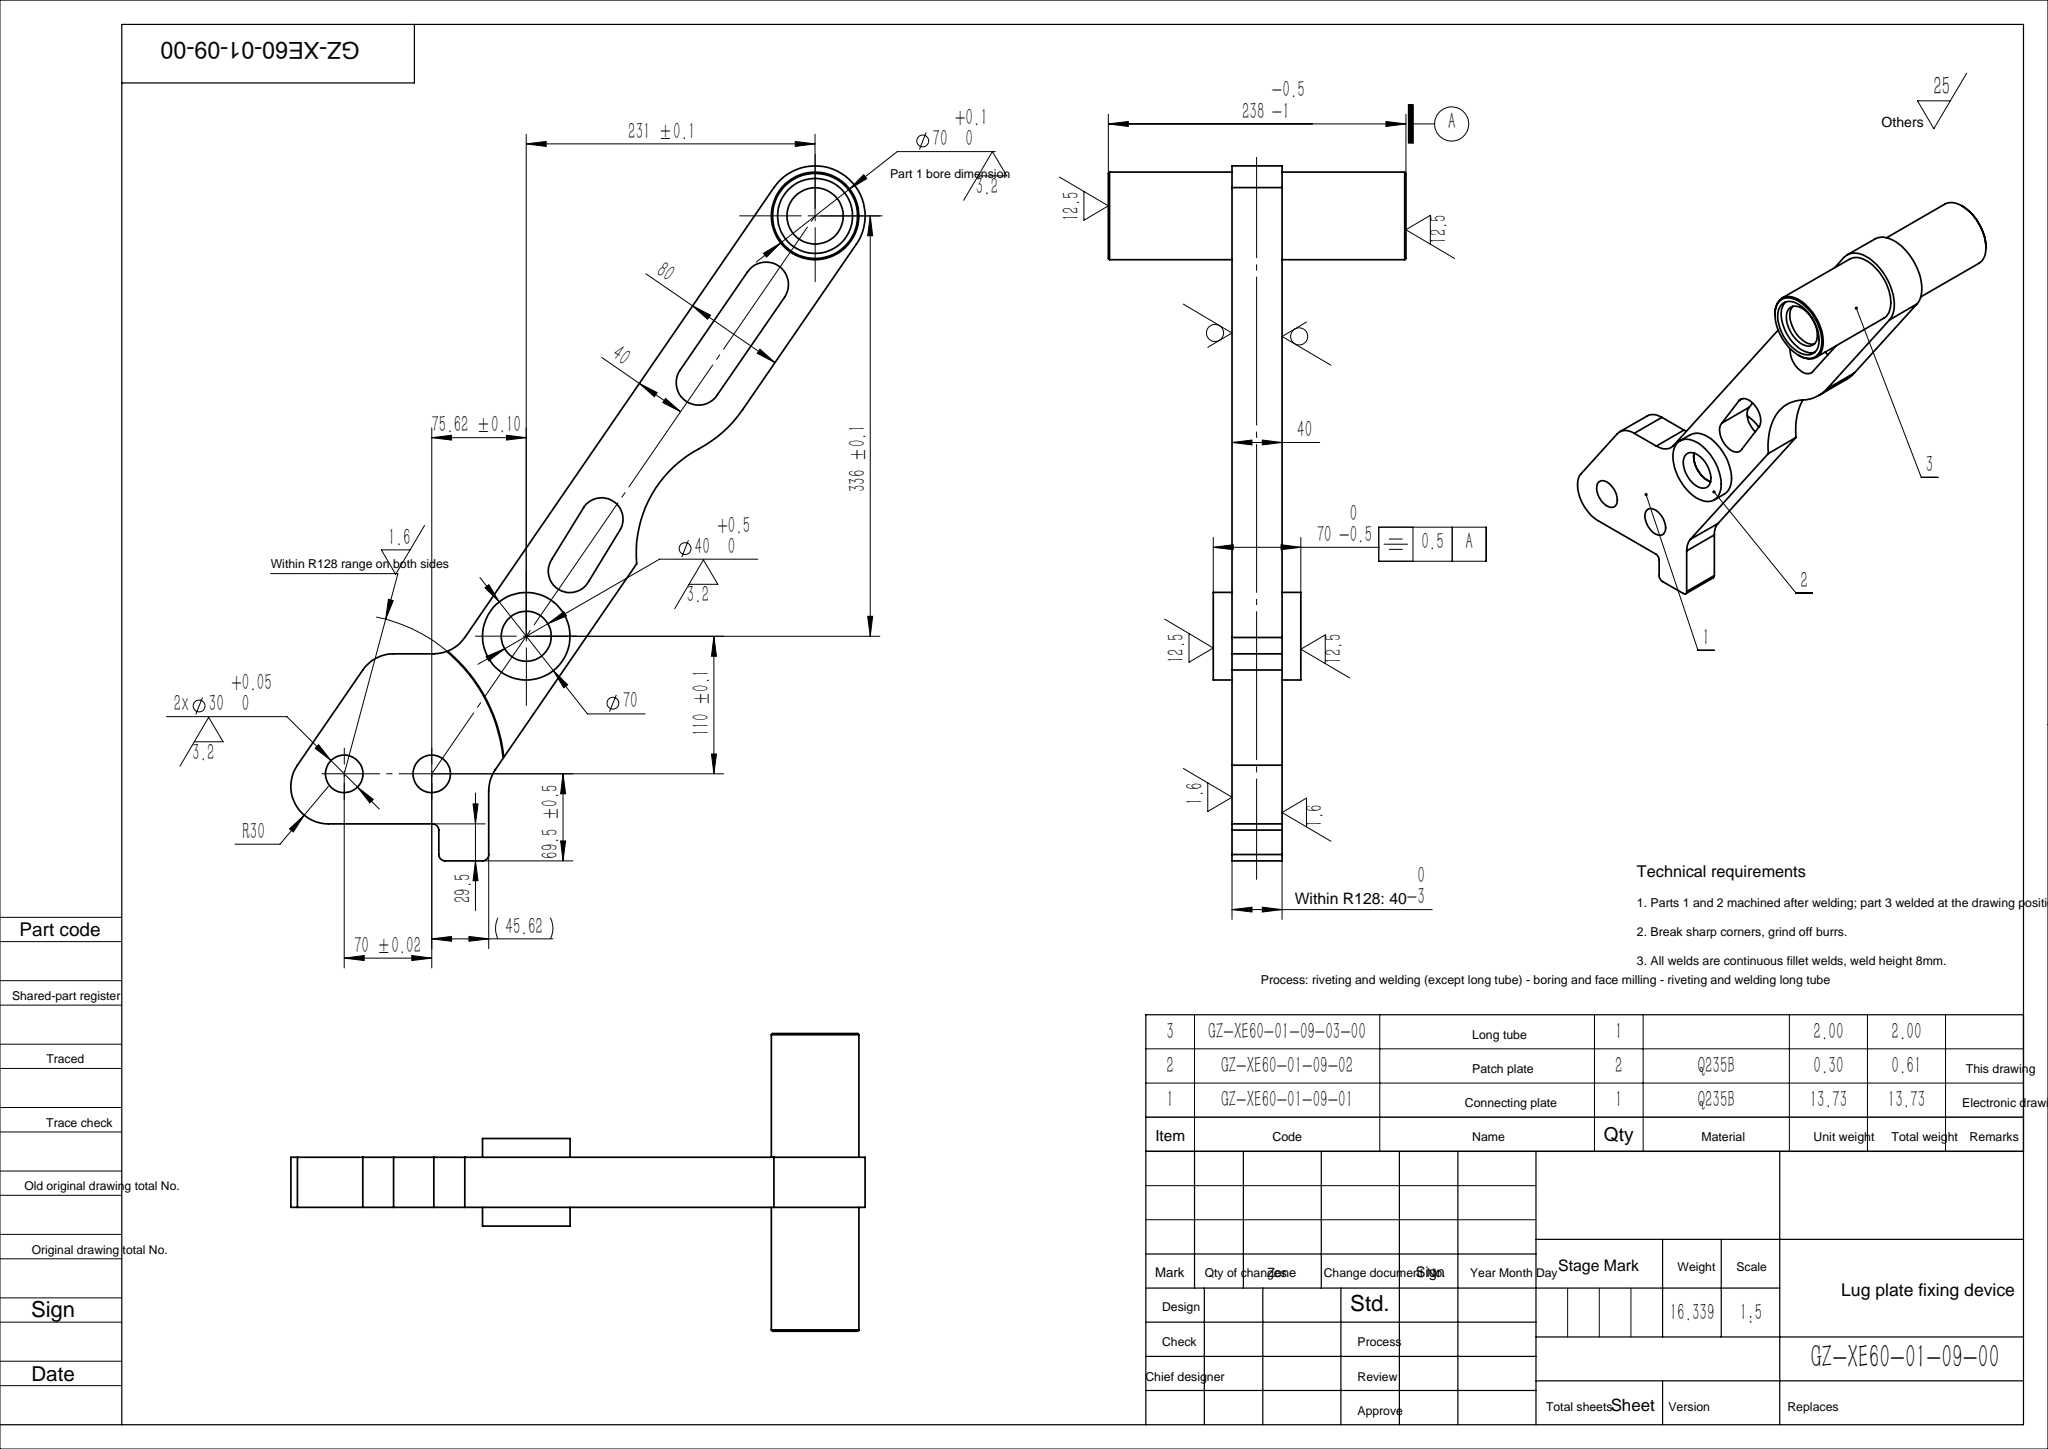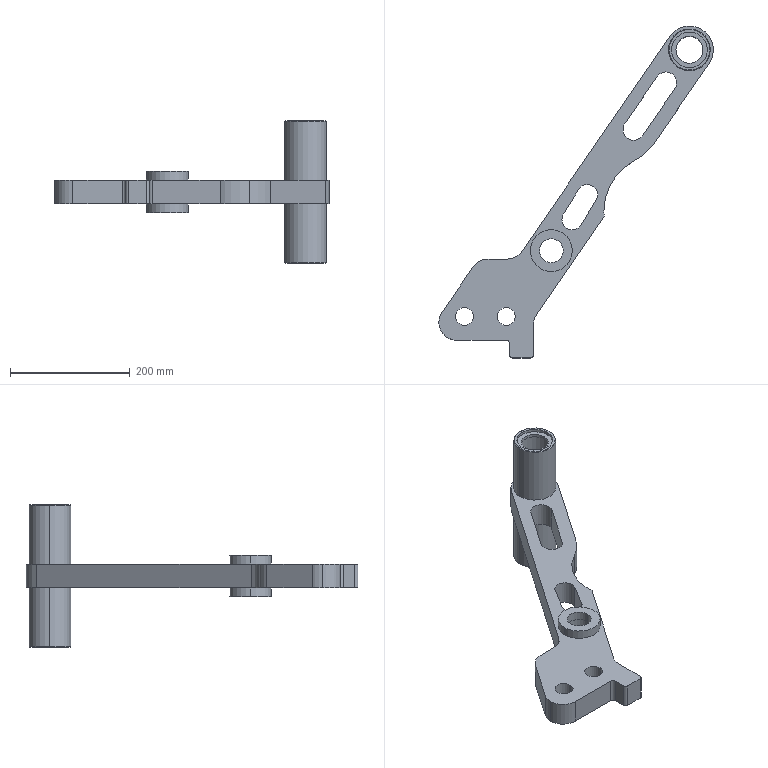Part | SolidWorks | 6 solids | 75 faces | box 459.333 x 555.5 x 238 mm | volume 2086739 mm3 | cylinder 46 | plane 25 | cone 4 | commonest cylinder face diameters 60 x11 70 x8 40 x6 30 x4 45 x4 10 x3